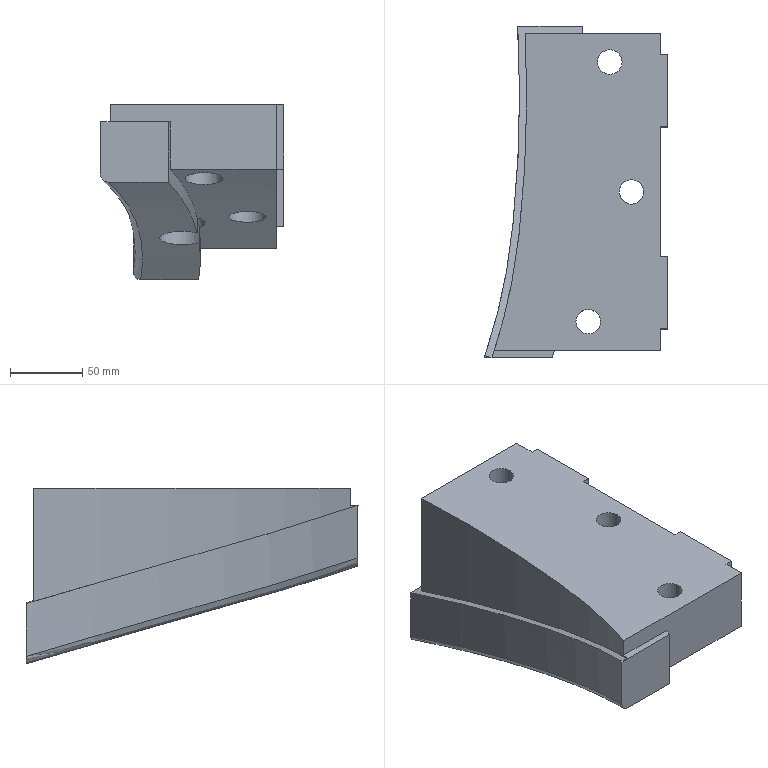Part | NX | features solid 2 | 1 solid | 36 faces | box 126.909 x 230 x 121.577 mm | volume 1727505 mm3 | plane 21 | spline 8 | cylinder 7 | commonest cylinder face diameters 17 x3 26 x3 32 x1